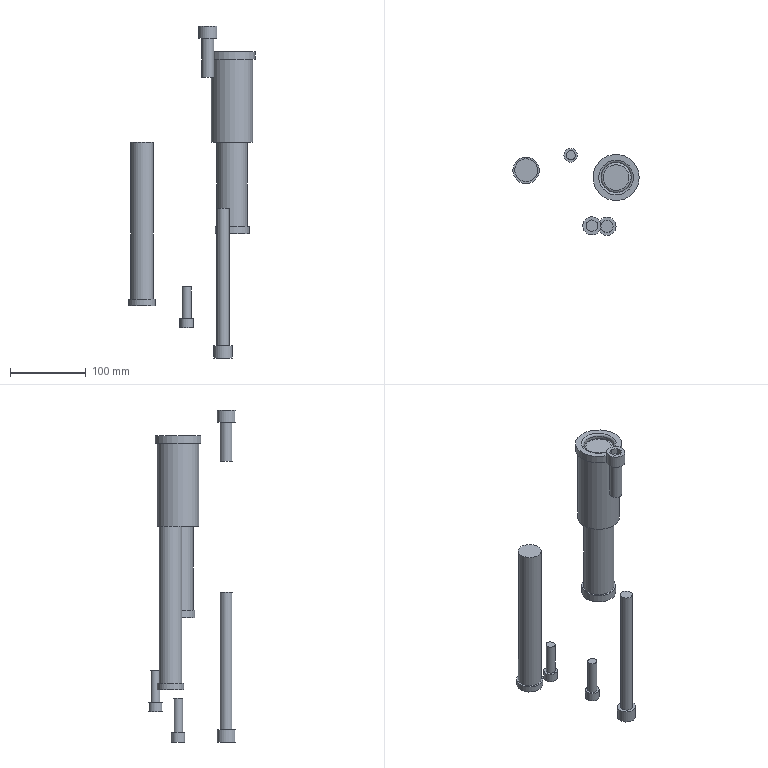Part | STEP file | MPPJ | 7 solids | 71 faces | box 167 x 115 x 439 mm | volume 666925 mm3 | plane 49 | cylinder 17 | torus 5 | commonest cylinder face diameters 40 x4 12 x2 16 x2 18 x2 24 x2 30 x1